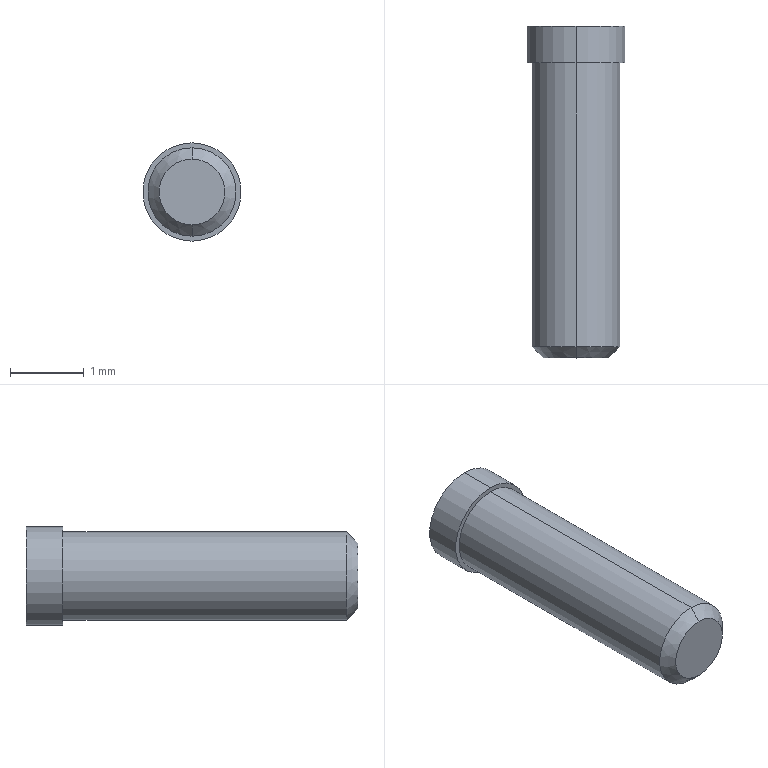Part | STEP file | MG_P_Screw_9_N | 1 solid | 16 faces | box 1.333 x 4.5 x 1.333 mm | volume 5.111 mm3 | plane 10 | cylinder 4 | cone 2 | commonest cylinder face diameters 1.2 x2 1.333 x2
STEP:
#1=CARTESIAN_POINT('',(0.,0.,0.));
#2=DIRECTION('',(0.,0.,1.));
#3=DIRECTION('',(1.,0.,0.));
#4=AXIS2_PLACEMENT_3D('',#1,#2,#3);
#5=CARTESIAN_POINT('',(0.,-4.,0.4465));
#6=VERTEX_POINT('',#5);
#7=CARTESIAN_POINT('',(0.,-4.,-0.4465));
#8=VERTEX_POINT('',#7);
#9=CARTESIAN_POINT('',(0.,-4.,0.));
#10=DIRECTION('',(0.,1.,0.));
#11=DIRECTION('',(0.,0.,1.));
#12=AXIS2_PLACEMENT_3D('',#9,#10,#11);
#13=CIRCLE('',#12,0.4465);
#14=CARTESIAN_POINT('',(0.,-4.,0.));
#15=DIRECTION('',(0.,1.,0.));
#16=DIRECTION('',(0.,0.,1.));
#17=AXIS2_PLACEMENT_3D('',#14,#15,#16);
#18=CONICAL_SURFACE('',#17,0.4465,0.7854);
#19=CARTESIAN_POINT('',(0.,0.));
#20=DIRECTION('',(1.,0.));
#21=VECTOR('',#20,1.);
#22=LINE('',#19,#21);
#23=(GEOMETRIC_REPRESENTATION_CONTEXT(2)PARAMETRIC_REPRESENTATION_CONTEXT()REPRESENTATION_CONTEXT('',''));
#24=DEFINITIONAL_REPRESENTATION('',(#22),#23);
#25=PCURVE('',#18,#24);
#26=CARTESIAN_POINT('',(0.4465,-4.,0.));
#27=DIRECTION('',(0.,1.,0.));
#28=DIRECTION('',(0.,0.,1.));
#29=AXIS2_PLACEMENT_3D('',#26,#27,#28);
#30=PLANE('',#29);
#31=CARTESIAN_POINT('',(0.,-0.4465));
#32=DIRECTION('',(1.,0.));
#33=AXIS2_PLACEMENT_2D('',#31,#32);
#34=CIRCLE('',#33,0.4465);
#35=(GEOMETRIC_REPRESENTATION_CONTEXT(2)PARAMETRIC_REPRESENTATION_CONTEXT()REPRESENTATION_CONTEXT('',''));
#36=DEFINITIONAL_REPRESENTATION('',(#34),#35);
#37=PCURVE('',#30,#36);
#38=SURFACE_CURVE('',#13,(#25,#37),.PCURVE_S1.);
#39=EDGE_CURVE('',#6,#8,#38,.T.);
#40=ORIENTED_EDGE('',*,*,#39,.T.);
#41=CARTESIAN_POINT('',(0.,-3.846,-0.6));
#42=VERTEX_POINT('',#41);
#43=CARTESIAN_POINT('',(0.,-4.,-0.4465));
#44=DIRECTION('',(0.,0.7071,-0.7071));
#45=VECTOR('',#44,1.);
#46=LINE('',#43,#45);
#47=CARTESIAN_POINT('',(3.142,0.));
#48=DIRECTION('',(0.,1.));
#49=VECTOR('',#48,1.);
#50=LINE('',#47,#49);
#51=(GEOMETRIC_REPRESENTATION_CONTEXT(2)PARAMETRIC_REPRESENTATION_CONTEXT()REPRESENTATION_CONTEXT('',''));
#52=DEFINITIONAL_REPRESENTATION('',(#50),#51);
#53=PCURVE('',#18,#52);
#54=CARTESIAN_POINT('',(0.,-4.,0.));
#55=DIRECTION('',(0.,1.,0.));
#56=DIRECTION('',(0.,0.,1.));
#57=AXIS2_PLACEMENT_3D('',#54,#55,#56);
#58=CONICAL_SURFACE('',#57,0.4465,0.7854);
#59=CARTESIAN_POINT('',(3.142,0.));
#60=DIRECTION('',(0.,1.));
#61=VECTOR('',#60,1.);
#62=LINE('',#59,#61);
#63=(GEOMETRIC_REPRESENTATION_CONTEXT(2)PARAMETRIC_REPRESENTATION_CONTEXT()REPRESENTATION_CONTEXT('',''));
#64=DEFINITIONAL_REPRESENTATION('',(#62),#63);
#65=PCURVE('',#58,#64);
#66=SURFACE_CURVE('',#46,(#53,#65),.PCURVE_S1.);
#67=EDGE_CURVE('',#8,#42,#66,.T.);
#68=ORIENTED_EDGE('',*,*,#67,.T.);
#69=CARTESIAN_POINT('',(0.,-3.846,0.6));
#70=VERTEX_POINT('',#69);
#71=CARTESIAN_POINT('',(0.,-3.846,0.));
#72=DIRECTION('',(0.,1.,0.));
#73=DIRECTION('',(0.,0.,1.));
#74=AXIS2_PLACEMENT_3D('',#71,#72,#73);
#75=CIRCLE('',#74,0.6);
#76=CARTESIAN_POINT('',(0.,0.1535));
#77=DIRECTION('',(1.,0.));
#78=VECTOR('',#77,1.);
#79=LINE('',#76,#78);
#80=(GEOMETRIC_REPRESENTATION_CONTEXT(2)PARAMETRIC_REPRESENTATION_CONTEXT()REPRESENTATION_CONTEXT('',''));
#81=DEFINITIONAL_REPRESENTATION('',(#79),#80);
#82=PCURVE('',#18,#81);
#83=CARTESIAN_POINT('',(0.,-4.,0.));
#84=DIRECTION('',(0.,1.,0.));
#85=DIRECTION('',(0.,0.,1.));
#86=AXIS2_PLACEMENT_3D('',#83,#84,#85);
#87=CYLINDRICAL_SURFACE('',#86,0.6);
#88=CARTESIAN_POINT('',(0.,0.1535));
#89=DIRECTION('',(1.,0.));
#90=VECTOR('',#89,1.);
#91=LINE('',#88,#90);
#92=(GEOMETRIC_REPRESENTATION_CONTEXT(2)PARAMETRIC_REPRESENTATION_CONTEXT()REPRESENTATION_CONTEXT('',''));
#93=DEFINITIONAL_REPRESENTATION('',(#91),#92);
#94=PCURVE('',#87,#93);
#95=SURFACE_CURVE('',#75,(#82,#94),.PCURVE_S1.);
#96=EDGE_CURVE('',#70,#42,#95,.T.);
#97=ORIENTED_EDGE('',*,*,#96,.F.);
#98=CARTESIAN_POINT('',(0.,-4.,0.4465));
#99=DIRECTION('',(0.,0.7071,0.7071));
#100=VECTOR('',#99,1.);
#101=LINE('',#98,#100);
#102=CARTESIAN_POINT('',(0.,0.));
#103=DIRECTION('',(0.,1.));
#104=VECTOR('',#103,1.);
#105=LINE('',#102,#104);
#106=(GEOMETRIC_REPRESENTATION_CONTEXT(2)PARAMETRIC_REPRESENTATION_CONTEXT()REPRESENTATION_CONTEXT('',''));
#107=DEFINITIONAL_REPRESENTATION('',(#105),#106);
#108=PCURVE('',#18,#107);
#109=CARTESIAN_POINT('',(6.283,0.));
#110=DIRECTION('',(0.,1.));
#111=VECTOR('',#110,1.);
#112=LINE('',#109,#111);
#113=(GEOMETRIC_REPRESENTATION_CONTEXT(2)PARAMETRIC_REPRESENTATION_CONTEXT()REPRESENTATION_CONTEXT('',''));
#114=DEFINITIONAL_REPRESENTATION('',(#112),#113);
#115=PCURVE('',#58,#114);
#116=SURFACE_CURVE('',#101,(#108,#115),.PCURVE_S1.);
#117=EDGE_CURVE('',#6,#70,#116,.T.);
#118=ORIENTED_EDGE('',*,*,#117,.F.);
#119=EDGE_LOOP('',(#40,#68,#97,#118));
#120=FACE_BOUND('',#119,.T.);
#121=ADVANCED_FACE('',(#120),#18,.T.);
#122=ORIENTED_EDGE('',*,*,#96,.T.);
#123=CARTESIAN_POINT('',(0.,0.,-0.6));
#124=VERTEX_POINT('',#123);
#125=CARTESIAN_POINT('',(0.,-4.,-0.6));
#126=DIRECTION('',(0.,1.,0.));
#127=VECTOR('',#126,1.);
#128=LINE('',#125,#127);
#129=CARTESIAN_POINT('',(3.142,0.));
#130=DIRECTION('',(0.,1.));
#131=VECTOR('',#130,1.);
#132=LINE('',#129,#131);
#133=(GEOMETRIC_REPRESENTATION_CONTEXT(2)PARAMETRIC_REPRESENTATION_CONTEXT()REPRESENTATION_CONTEXT('',''));
#134=DEFINITIONAL_REPRESENTATION('',(#132),#133);
#135=PCURVE('',#87,#134);
#136=CARTESIAN_POINT('',(0.,-4.,0.));
#137=DIRECTION('',(0.,1.,0.));
#138=DIRECTION('',(0.,0.,1.));
#139=AXIS2_PLACEMENT_3D('',#136,#137,#138);
#140=CYLINDRICAL_SURFACE('',#139,0.6);
#141=CARTESIAN_POINT('',(3.142,0.));
#142=DIRECTION('',(0.,1.));
#143=VECTOR('',#142,1.);
#144=LINE('',#141,#143);
#145=(GEOMETRIC_REPRESENTATION_CONTEXT(2)PARAMETRIC_REPRESENTATION_CONTEXT()REPRESENTATION_CONTEXT('',''));
#146=DEFINITIONAL_REPRESENTATION('',(#144),#145);
#147=PCURVE('',#140,#146);
#148=SURFACE_CURVE('',#128,(#135,#147),.PCURVE_S1.);
#149=EDGE_CURVE('',#42,#124,#148,.T.);
#150=ORIENTED_EDGE('',*,*,#149,.T.);
#151=CARTESIAN_POINT('',(0.,0.,0.6));
#152=VERTEX_POINT('',#151);
#153=CARTESIAN_POINT('',(0.,0.,0.));
#154=DIRECTION('',(0.,1.,0.));
#155=DIRECTION('',(0.,0.,1.));
#156=AXIS2_PLACEMENT_3D('',#153,#154,#155);
#157=CIRCLE('',#156,0.6);
#158=CARTESIAN_POINT('',(0.,4.));
#159=DIRECTION('',(1.,0.));
#160=VECTOR('',#159,1.);
#161=LINE('',#158,#160);
#162=(GEOMETRIC_REPRESENTATION_CONTEXT(2)PARAMETRIC_REPRESENTATION_CONTEXT()REPRESENTATION_CONTEXT('',''));
#163=DEFINITIONAL_REPRESENTATION('',(#161),#162);
#164=PCURVE('',#87,#163);
#165=CARTESIAN_POINT('',(0.6667,0.,0.));
#166=DIRECTION('',(0.,1.,0.));
#167=DIRECTION('',(0.,0.,1.));
#168=AXIS2_PLACEMENT_3D('',#165,#166,#167);
#169=PLANE('',#168);
#170=CARTESIAN_POINT('',(0.,-0.6667));
#171=DIRECTION('',(1.,0.));
#172=AXIS2_PLACEMENT_2D('',#170,#171);
#173=CIRCLE('',#172,0.6);
#174=(GEOMETRIC_REPRESENTATION_CONTEXT(2)PARAMETRIC_REPRESENTATION_CONTEXT()REPRESENTATION_CONTEXT('',''));
#175=DEFINITIONAL_REPRESENTATION('',(#173),#174);
#176=PCURVE('',#169,#175);
#177=SURFACE_CURVE('',#157,(#164,#176),.PCURVE_S1.);
#178=EDGE_CURVE('',#152,#124,#177,.T.);
#179=ORIENTED_EDGE('',*,*,#178,.F.);
#180=CARTESIAN_POINT('',(0.,-4.,0.6));
#181=DIRECTION('',(0.,1.,0.));
#182=VECTOR('',#181,1.);
#183=LINE('',#180,#182);
#184=CARTESIAN_POINT('',(0.,0.));
#185=DIRECTION('',(0.,1.));
#186=VECTOR('',#185,1.);
#187=LINE('',#184,#186);
#188=(GEOMETRIC_REPRESENTATION_CONTEXT(2)PARAMETRIC_REPRESENTATION_CONTEXT()REPRESENTATION_CONTEXT('',''));
#189=DEFINITIONAL_REPRESENTATION('',(#187),#188);
#190=PCURVE('',#87,#189);
#191=CARTESIAN_POINT('',(6.283,0.));
#192=DIRECTION('',(0.,1.));
#193=VECTOR('',#192,1.);
#194=LINE('',#191,#193);
#195=(GEOMETRIC_REPRESENTATION_CONTEXT(2)PARAMETRIC_REPRESENTATION_CONTEXT()REPRESENTATION_CONTEXT('',''));
#196=DEFINITIONAL_REPRESENTATION('',(#194),#195);
#197=PCURVE('',#140,#196);
#198=SURFACE_CURVE('',#183,(#190,#197),.PCURVE_S1.);
#199=EDGE_CURVE('',#70,#152,#198,.T.);
#200=ORIENTED_EDGE('',*,*,#199,.F.);
#201=EDGE_LOOP('',(#122,#150,#179,#200));
#202=FACE_BOUND('',#201,.T.);
#203=ADVANCED_FACE('',(#202),#87,.T.);
#204=CARTESIAN_POINT('',(0.,0.,0.6667));
#205=VERTEX_POINT('',#204);
#206=CARTESIAN_POINT('',(0.,0.,-0.6667));
#207=VERTEX_POINT('',#206);
#208=CARTESIAN_POINT('',(0.,0.,0.));
#209=DIRECTION('',(0.,1.,0.));
#210=DIRECTION('',(0.,0.,1.));
#211=AXIS2_PLACEMENT_3D('',#208,#209,#210);
#212=CIRCLE('',#211,0.6667);
#213=CARTESIAN_POINT('',(0.,-4.,0.));
#214=DIRECTION('',(0.,1.,0.));
#215=DIRECTION('',(0.,0.,1.));
#216=AXIS2_PLACEMENT_3D('',#213,#214,#215);
#217=CYLINDRICAL_SURFACE('',#216,0.6667);
#218=CARTESIAN_POINT('',(0.,4.));
#219=DIRECTION('',(1.,0.));
#220=VECTOR('',#219,1.);
#221=LINE('',#218,#220);
#222=(GEOMETRIC_REPRESENTATION_CONTEXT(2)PARAMETRIC_REPRESENTATION_CONTEXT()REPRESENTATION_CONTEXT('',''));
#223=DEFINITIONAL_REPRESENTATION('',(#221),#222);
#224=PCURVE('',#217,#223);
#225=CARTESIAN_POINT('',(0.,-0.6667));
#226=DIRECTION('',(1.,0.));
#227=AXIS2_PLACEMENT_2D('',#225,#226);
#228=CIRCLE('',#227,0.6667);
#229=(GEOMETRIC_REPRESENTATION_CONTEXT(2)PARAMETRIC_REPRESENTATION_CONTEXT()REPRESENTATION_CONTEXT('',''));
#230=DEFINITIONAL_REPRESENTATION('',(#228),#229);
#231=PCURVE('',#169,#230);
#232=SURFACE_CURVE('',#212,(#224,#231),.PCURVE_S1.);
#233=EDGE_CURVE('',#205,#207,#232,.T.);
#234=ORIENTED_EDGE('',*,*,#233,.T.);
#235=CARTESIAN_POINT('',(0.,0.5,-0.6667));
#236=VERTEX_POINT('',#235);
#237=CARTESIAN_POINT('',(0.,-4.,-0.6667));
#238=DIRECTION('',(0.,1.,0.));
#239=VECTOR('',#238,1.);
#240=LINE('',#237,#239);
#241=CARTESIAN_POINT('',(3.142,0.));
#242=DIRECTION('',(0.,1.));
#243=VECTOR('',#242,1.);
#244=LINE('',#241,#243);
#245=(GEOMETRIC_REPRESENTATION_CONTEXT(2)PARAMETRIC_REPRESENTATION_CONTEXT()REPRESENTATION_CONTEXT('',''));
#246=DEFINITIONAL_REPRESENTATION('',(#244),#245);
#247=PCURVE('',#217,#246);
#248=CARTESIAN_POINT('',(0.,-4.,0.));
#249=DIRECTION('',(0.,1.,0.));
#250=DIRECTION('',(0.,0.,1.));
#251=AXIS2_PLACEMENT_3D('',#248,#249,#250);
#252=CYLINDRICAL_SURFACE('',#251,0.6667);
#253=CARTESIAN_POINT('',(3.142,0.));
#254=DIRECTION('',(0.,1.));
#255=VECTOR('',#254,1.);
#256=LINE('',#253,#255);
#257=(GEOMETRIC_REPRESENTATION_CONTEXT(2)PARAMETRIC_REPRESENTATION_CONTEXT()REPRESENTATION_CONTEXT('',''));
#258=DEFINITIONAL_REPRESENTATION('',(#256),#257);
#259=PCURVE('',#252,#258);
#260=SURFACE_CURVE('',#240,(#247,#259),.PCURVE_S1.);
#261=EDGE_CURVE('',#207,#236,#260,.T.);
#262=ORIENTED_EDGE('',*,*,#261,.T.);
#263=CARTESIAN_POINT('',(0.,0.5,0.6667));
#264=VERTEX_POINT('',#263);
#265=CARTESIAN_POINT('',(0.,0.5,0.));
#266=DIRECTION('',(0.,1.,0.));
#267=DIRECTION('',(0.,0.,1.));
#268=AXIS2_PLACEMENT_3D('',#265,#266,#267);
#269=CIRCLE('',#268,0.6667);
#270=CARTESIAN_POINT('',(0.,4.5));
#271=DIRECTION('',(1.,0.));
#272=VECTOR('',#271,1.);
#273=LINE('',#270,#272);
#274=(GEOMETRIC_REPRESENTATION_CONTEXT(2)PARAMETRIC_REPRESENTATION_CONTEXT()REPRESENTATION_CONTEXT('',''));
#275=DEFINITIONAL_REPRESENTATION('',(#273),#274);
#276=PCURVE('',#217,#275);
#277=CARTESIAN_POINT('',(0.,0.5,0.));
#278=DIRECTION('',(0.,-1.,0.));
#279=DIRECTION('',(0.,0.,-1.));
#280=AXIS2_PLACEMENT_3D('',#277,#278,#279);
#281=PLANE('',#280);
#282=CARTESIAN_POINT('',(-0.6667,0.));
#283=CARTESIAN_POINT('',(-0.6667,1.155));
#284=CARTESIAN_POINT('',(0.3333,0.5774));
#285=CARTESIAN_POINT('',(1.333,0.));
#286=CARTESIAN_POINT('',(0.3333,-0.5774));
#287=CARTESIAN_POINT('',(-0.6667,-1.155));
#288=CARTESIAN_POINT('',(-0.6667,0.));
#289=(BOUNDED_CURVE()B_SPLINE_CURVE(2,(#282,#283,#284,#285,#286,#287,#288),.UNSPECIFIED.,.T.,.F.)B_SPLINE_CURVE_WITH_KNOTS((1,2,2,2,2,1),(-2.094,0.,2.094,4.189,6.283,8.378),.UNSPECIFIED.)CURVE()GEOMETRIC_REPRESENTATION_ITEM()RATIONAL_B_SPLINE_CURVE((1.,0.5,1.,0.5,1.,0.5,1.))REPRESENTATION_ITEM(''));
#290=(GEOMETRIC_REPRESENTATION_CONTEXT(2)PARAMETRIC_REPRESENTATION_CONTEXT()REPRESENTATION_CONTEXT('',''));
#291=DEFINITIONAL_REPRESENTATION('',(#289),#290);
#292=PCURVE('',#281,#291);
#293=SURFACE_CURVE('',#269,(#276,#292),.PCURVE_S1.);
#294=EDGE_CURVE('',#264,#236,#293,.T.);
#295=ORIENTED_EDGE('',*,*,#294,.F.);
#296=CARTESIAN_POINT('',(0.,-4.,0.6667));
#297=DIRECTION('',(0.,1.,0.));
#298=VECTOR('',#297,1.);
#299=LINE('',#296,#298);
#300=CARTESIAN_POINT('',(0.,0.));
#301=DIRECTION('',(0.,1.));
#302=VECTOR('',#301,1.);
#303=LINE('',#300,#302);
#304=(GEOMETRIC_REPRESENTATION_CONTEXT(2)PARAMETRIC_REPRESENTATION_CONTEXT()REPRESENTATION_CONTEXT('',''));
#305=DEFINITIONAL_REPRESENTATION('',(#303),#304);
#306=PCURVE('',#217,#305);
#307=CARTESIAN_POINT('',(6.283,0.));
#308=DIRECTION('',(0.,1.));
#309=VECTOR('',#308,1.);
#310=LINE('',#307,#309);
#311=(GEOMETRIC_REPRESENTATION_CONTEXT(2)PARAMETRIC_REPRESENTATION_CONTEXT()REPRESENTATION_CONTEXT('',''));
#312=DEFINITIONAL_REPRESENTATION('',(#310),#311);
#313=PCURVE('',#252,#312);
#314=SURFACE_CURVE('',#299,(#306,#313),.PCURVE_S1.);
#315=EDGE_CURVE('',#205,#264,#314,.T.);
#316=ORIENTED_EDGE('',*,*,#315,.F.);
#317=EDGE_LOOP('',(#234,#262,#295,#316));
#318=FACE_BOUND('',#317,.T.);
#319=ADVANCED_FACE('',(#318),#217,.T.);
#320=CARTESIAN_POINT('',(-0.2857,0.5,0.165));
#321=VERTEX_POINT('',#320);
#322=CARTESIAN_POINT('',(0.,0.5,0.3299));
#323=VERTEX_POINT('',#322);
#324=CARTESIAN_POINT('',(-0.2857,0.5,0.165));
#325=DIRECTION('',(0.866,0.,0.5));
#326=VECTOR('',#325,1.);
#327=LINE('',#324,#326);
#328=CARTESIAN_POINT('',(-0.165,-0.2857));
#329=DIRECTION('',(-0.5,0.866));
#330=VECTOR('',#329,1.);
#331=LINE('',#328,#330);
#332=(GEOMETRIC_REPRESENTATION_CONTEXT(2)PARAMETRIC_REPRESENTATION_CONTEXT()REPRESENTATION_CONTEXT('',''));
#333=DEFINITIONAL_REPRESENTATION('',(#331),#332);
#334=PCURVE('',#281,#333);
#335=CARTESIAN_POINT('',(-0.2857,0.25,0.165));
#336=DIRECTION('',(-0.5,0.,0.866));
#337=DIRECTION('',(0.866,0.,0.5));
#338=AXIS2_PLACEMENT_3D('',#335,#336,#337);
#339=PLANE('',#338);
#340=CARTESIAN_POINT('',(0.,0.25));
#341=DIRECTION('',(1.,0.));
#342=VECTOR('',#341,1.);
#343=LINE('',#340,#342);
#344=(GEOMETRIC_REPRESENTATION_CONTEXT(2)PARAMETRIC_REPRESENTATION_CONTEXT()REPRESENTATION_CONTEXT('',''));
#345=DEFINITIONAL_REPRESENTATION('',(#343),#344);
#346=PCURVE('',#339,#345);
#347=SURFACE_CURVE('',#327,(#334,#346),.PCURVE_S1.);
#348=EDGE_CURVE('',#321,#323,#347,.T.);
#349=ORIENTED_EDGE('',*,*,#348,.F.);
#350=CARTESIAN_POINT('',(-0.2857,0.5,-0.165));
#351=VERTEX_POINT('',#350);
#352=CARTESIAN_POINT('',(-0.2857,0.5,-0.165));
#353=DIRECTION('',(0.,0.,1.));
#354=VECTOR('',#353,1.);
#355=LINE('',#352,#354);
#356=CARTESIAN_POINT('',(0.165,-0.2857));
#357=DIRECTION('',(-1.,0.));
#358=VECTOR('',#357,1.);
#359=LINE('',#356,#358);
#360=(GEOMETRIC_REPRESENTATION_CONTEXT(2)PARAMETRIC_REPRESENTATION_CONTEXT()REPRESENTATION_CONTEXT('',''));
#361=DEFINITIONAL_REPRESENTATION('',(#359),#360);
#362=PCURVE('',#281,#361);
#363=CARTESIAN_POINT('',(-0.2857,0.25,-0.165));
#364=DIRECTION('',(-1.,0.,0.));
#365=DIRECTION('',(0.,0.,1.));
#366=AXIS2_PLACEMENT_3D('',#363,#364,#365);
#367=PLANE('',#366);
#368=CARTESIAN_POINT('',(0.,0.25));
#369=DIRECTION('',(1.,0.));
#370=VECTOR('',#369,1.);
#371=LINE('',#368,#370);
#372=(GEOMETRIC_REPRESENTATION_CONTEXT(2)PARAMETRIC_REPRESENTATION_CONTEXT()REPRESENTATION_CONTEXT('',''));
#373=DEFINITIONAL_REPRESENTATION('',(#371),#372);
#374=PCURVE('',#367,#373);
#375=SURFACE_CURVE('',#355,(#362,#374),.PCURVE_S1.);
#376=EDGE_CURVE('',#351,#321,#375,.T.);
#377=ORIENTED_EDGE('',*,*,#376,.F.);
#378=CARTESIAN_POINT('',(0.,0.5,-0.3299));
#379=VERTEX_POINT('',#378);
#380=CARTESIAN_POINT('',(0.,0.5,-0.3299));
#381=DIRECTION('',(-0.866,0.,0.5));
#382=VECTOR('',#381,1.);
#383=LINE('',#380,#382);
#384=CARTESIAN_POINT('',(0.3299,0.));
#385=DIRECTION('',(-0.5,-0.866));
#386=VECTOR('',#385,1.);
#387=LINE('',#384,#386);
#388=(GEOMETRIC_REPRESENTATION_CONTEXT(2)PARAMETRIC_REPRESENTATION_CONTEXT()REPRESENTATION_CONTEXT('',''));
#389=DEFINITIONAL_REPRESENTATION('',(#387),#388);
#390=PCURVE('',#281,#389);
#391=CARTESIAN_POINT('',(0.,0.25,-0.3299));
#392=DIRECTION('',(-0.5,0.,-0.866));
#393=DIRECTION('',(-0.866,0.,0.5));
#394=AXIS2_PLACEMENT_3D('',#391,#392,#393);
#395=PLANE('',#394);
#396=CARTESIAN_POINT('',(0.,0.25));
#397=DIRECTION('',(1.,0.));
#398=VECTOR('',#397,1.);
#399=LINE('',#396,#398);
#400=(GEOMETRIC_REPRESENTATION_CONTEXT(2)PARAMETRIC_REPRESENTATION_CONTEXT()REPRESENTATION_CONTEXT('',''));
#401=DEFINITIONAL_REPRESENTATION('',(#399),#400);
#402=PCURVE('',#395,#401);
#403=SURFACE_CURVE('',#383,(#390,#402),.PCURVE_S1.);
#404=EDGE_CURVE('',#379,#351,#403,.T.);
#405=ORIENTED_EDGE('',*,*,#404,.F.);
#406=CARTESIAN_POINT('',(0.2857,0.5,-0.165));
#407=VERTEX_POINT('',#406);
#408=CARTESIAN_POINT('',(0.2857,0.5,-0.165));
#409=DIRECTION('',(-0.866,0.,-0.5));
#410=VECTOR('',#409,1.);
#411=LINE('',#408,#410);
#412=CARTESIAN_POINT('',(0.165,0.2857));
#413=DIRECTION('',(0.5,-0.866));
#414=VECTOR('',#413,1.);
#415=LINE('',#412,#414);
#416=(GEOMETRIC_REPRESENTATION_CONTEXT(2)PARAMETRIC_REPRESENTATION_CONTEXT()REPRESENTATION_CONTEXT('',''));
#417=DEFINITIONAL_REPRESENTATION('',(#415),#416);
#418=PCURVE('',#281,#417);
#419=CARTESIAN_POINT('',(0.2857,0.25,-0.165));
#420=DIRECTION('',(0.5,0.,-0.866));
#421=DIRECTION('',(-0.866,0.,-0.5));
#422=AXIS2_PLACEMENT_3D('',#419,#420,#421);
#423=PLANE('',#422);
#424=CARTESIAN_POINT('',(0.,0.25));
#425=DIRECTION('',(1.,0.));
#426=VECTOR('',#425,1.);
#427=LINE('',#424,#426);
#428=(GEOMETRIC_REPRESENTATION_CONTEXT(2)PARAMETRIC_REPRESENTATION_CONTEXT()REPRESENTATION_CONTEXT('',''));
#429=DEFINITIONAL_REPRESENTATION('',(#427),#428);
#430=PCURVE('',#423,#429);
#431=SURFACE_CURVE('',#411,(#418,#430),.PCURVE_S1.);
#432=EDGE_CURVE('',#407,#379,#431,.T.);
#433=ORIENTED_EDGE('',*,*,#432,.F.);
#434=CARTESIAN_POINT('',(0.2857,0.5,0.165));
#435=VERTEX_POINT('',#434);
#436=CARTESIAN_POINT('',(0.2857,0.5,0.165));
#437=DIRECTION('',(0.,0.,-1.));
#438=VECTOR('',#437,1.);
#439=LINE('',#436,#438);
#440=CARTESIAN_POINT('',(-0.165,0.2857));
#441=DIRECTION('',(1.,0.));
#442=VECTOR('',#441,1.);
#443=LINE('',#440,#442);
#444=(GEOMETRIC_REPRESENTATION_CONTEXT(2)PARAMETRIC_REPRESENTATION_CONTEXT()REPRESENTATION_CONTEXT('',''));
#445=DEFINITIONAL_REPRESENTATION('',(#443),#444);
#446=PCURVE('',#281,#445);
#447=CARTESIAN_POINT('',(0.2857,0.25,0.165));
#448=DIRECTION('',(1.,0.,0.));
#449=DIRECTION('',(0.,0.,-1.));
#450=AXIS2_PLACEMENT_3D('',#447,#448,#449);
#451=PLANE('',#450);
#452=CARTESIAN_POINT('',(0.,0.25));
#453=DIRECTION('',(1.,0.));
#454=VECTOR('',#453,1.);
#455=LINE('',#452,#454);
#456=(GEOMETRIC_REPRESENTATION_CONTEXT(2)PARAMETRIC_REPRESENTATION_CONTEXT()REPRESENTATION_CONTEXT('',''));
#457=DEFINITIONAL_REPRESENTATION('',(#455),#456);
#458=PCURVE('',#451,#457);
#459=SURFACE_CURVE('',#439,(#446,#458),.PCURVE_S1.);
#460=EDGE_CURVE('',#435,#407,#459,.T.);
#461=ORIENTED_EDGE('',*,*,#460,.F.);
#462=CARTESIAN_POINT('',(0.,0.5,0.3299));
#463=DIRECTION('',(0.866,0.,-0.5));
#464=VECTOR('',#463,1.);
#465=LINE('',#462,#464);
#466=CARTESIAN_POINT('',(-0.3299,0.));
#467=DIRECTION('',(0.5,0.866));
#468=VECTOR('',#467,1.);
#469=LINE('',#466,#468);
#470=(GEOMETRIC_REPRESENTATION_CONTEXT(2)PARAMETRIC_REPRESENTATION_CONTEXT()REPRESENTATION_CONTEXT('',''));
#471=DEFINITIONAL_REPRESENTATION('',(#469),#470);
#472=PCURVE('',#281,#471);
#473=CARTESIAN_POINT('',(0.,0.25,0.3299));
#474=DIRECTION('',(0.5,0.,0.866));
#475=DIRECTION('',(0.866,0.,-0.5));
#476=AXIS2_PLACEMENT_3D('',#473,#474,#475);
#477=PLANE('',#476);
#478=CARTESIAN_POINT('',(0.,0.25));
#479=DIRECTION('',(1.,0.));
#480=VECTOR('',#479,1.);
#481=LINE('',#478,#480);
#482=(GEOMETRIC_REPRESENTATION_CONTEXT(2)PARAMETRIC_REPRESENTATION_CONTEXT()REPRESENTATION_CONTEXT('',''));
#483=DEFINITIONAL_REPRESENTATION('',(#481),#482);
#484=PCURVE('',#477,#483);
#485=SURFACE_CURVE('',#465,(#472,#484),.PCURVE_S1.);
#486=EDGE_CURVE('',#323,#435,#485,.T.);
#487=ORIENTED_EDGE('',*,*,#486,.F.);
#488=EDGE_LOOP('',(#349,#377,#405,#433,#461,#487));
#489=FACE_BOUND('',#488,.T.);
#490=ORIENTED_EDGE('',*,*,#294,.T.);
#491=CARTESIAN_POINT('',(0.,0.5,0.));
#492=DIRECTION('',(0.,1.,0.));
#493=DIRECTION('',(0.,0.,1.));
#494=AXIS2_PLACEMENT_3D('',#491,#492,#493);
#495=CIRCLE('',#494,0.6667);
#496=CARTESIAN_POINT('',(-0.6667,0.));
#497=CARTESIAN_POINT('',(-0.6667,1.155));
#498=CARTESIAN_POINT('',(0.3333,0.5774));
#499=CARTESIAN_POINT('',(1.333,0.));
#500=CARTESIAN_POINT('',(0.3333,-0.5774));
#501=CARTESIAN_POINT('',(-0.6667,-1.155));
#502=CARTESIAN_POINT('',(-0.6667,0.));
#503=(BOUNDED_CURVE()B_SPLINE_CURVE(2,(#496,#497,#498,#499,#500,#501,#502),.UNSPECIFIED.,.T.,.F.)B_SPLINE_CURVE_WITH_KNOTS((1,2,2,2,2,1),(-2.094,0.,2.094,4.189,6.283,8.378),.UNSPECIFIED.)CURVE()GEOMETRIC_REPRESENTATION_ITEM()RATIONAL_B_SPLINE_CURVE((1.,0.5,1.,0.5,1.,0.5,1.))REPRESENTATION_ITEM(''));
#504=(GEOMETRIC_REPRESENTATION_CONTEXT(2)PARAMETRIC_REPRESENTATION_CONTEXT()REPRESENTATION_CONTEXT('',''));
#505=DEFINITIONAL_REPRESENTATION('',(#503),#504);
#506=PCURVE('',#281,#505);
#507=CARTESIAN_POINT('',(0.,4.5));
#508=DIRECTION('',(1.,0.));
#509=VECTOR('',#508,1.);
#510=LINE('',#507,#509);
#511=(GEOMETRIC_REPRESENTATION_CONTEXT(2)PARAMETRIC_REPRESENTATION_CONTEXT()REPRESENTATION_CONTEXT('',''));
#512=DEFINITIONAL_REPRESENTATION('',(#510),#511);
#513=PCURVE('',#252,#512);
#514=SURFACE_CURVE('',#495,(#506,#513),.PCURVE_S1.);
#515=EDGE_CURVE('',#236,#264,#514,.T.);
#516=ORIENTED_EDGE('',*,*,#515,.T.);
#517=EDGE_LOOP('',(#490,#516));
#518=FACE_BOUND('',#517,.T.);
#519=ADVANCED_FACE('',(#489,#518),#281,.F.);
#520=ORIENTED_EDGE('',*,*,#261,.F.);
#521=CARTESIAN_POINT('',(0.,0.,0.));
#522=DIRECTION('',(0.,1.,0.));
#523=DIRECTION('',(0.,0.,1.));
#524=AXIS2_PLACEMENT_3D('',#521,#522,#523);
#525=CIRCLE('',#524,0.6667);
#526=CARTESIAN_POINT('',(0.,4.));
#527=DIRECTION('',(1.,0.));
#528=VECTOR('',#527,1.);
#529=LINE('',#526,#528);
#530=(GEOMETRIC_REPRESENTATION_CONTEXT(2)PARAMETRIC_REPRESENTATION_CONTEXT()REPRESENTATION_CONTEXT('',''));
#531=DEFINITIONAL_REPRESENTATION('',(#529),#530);
#532=PCURVE('',#252,#531);
#533=CARTESIAN_POINT('',(0.,-0.6667));
#534=DIRECTION('',(1.,0.));
#535=AXIS2_PLACEMENT_2D('',#533,#534);
#536=CIRCLE('',#535,0.6667);
#537=(GEOMETRIC_REPRESENTATION_CONTEXT(2)PARAMETRIC_REPRESENTATION_CONTEXT()REPRESENTATION_CONTEXT('',''));
#538=DEFINITIONAL_REPRESENTATION('',(#536),#537);
#539=PCURVE('',#169,#538);
#540=SURFACE_CURVE('',#525,(#532,#539),.PCURVE_S1.);
#541=EDGE_CURVE('',#207,#205,#540,.T.);
#542=ORIENTED_EDGE('',*,*,#541,.T.);
#543=ORIENTED_EDGE('',*,*,#315,.T.);
#544=ORIENTED_EDGE('',*,*,#515,.F.);
#545=EDGE_LOOP('',(#520,#542,#543,#544));
#546=FACE_BOUND('',#545,.T.);
#547=ADVANCED_FACE('',(#546),#252,.T.);
#548=ORIENTED_EDGE('',*,*,#233,.F.);
#549=ORIENTED_EDGE('',*,*,#541,.F.);
#550=EDGE_LOOP('',(#548,#549));
#551=FACE_BOUND('',#550,.T.);
#552=ORIENTED_EDGE('',*,*,#178,.T.);
#553=CARTESIAN_POINT('',(0.,0.,0.));
#554=DIRECTION('',(0.,1.,0.));
#555=DIRECTION('',(0.,0.,1.));
#556=AXIS2_PLACEMENT_3D('',#553,#554,#555);
#557=CIRCLE('',#556,0.6);
#558=CARTESIAN_POINT('',(0.,-0.6667));
#559=DIRECTION('',(1.,0.));
#560=AXIS2_PLACEMENT_2D('',#558,#559);
#561=CIRCLE('',#560,0.6);
#562=(GEOMETRIC_REPRESENTATION_CONTEXT(2)PARAMETRIC_REPRESENTATION_CONTEXT()REPRESENTATION_CONTEXT('',''));
#563=DEFINITIONAL_REPRESENTATION('',(#561),#562);
#564=PCURVE('',#169,#563);
#565=CARTESIAN_POINT('',(0.,4.));
#566=DIRECTION('',(1.,0.));
#567=VECTOR('',#566,1.);
#568=LINE('',#565,#567);
#569=(GEOMETRIC_REPRESENTATION_CONTEXT(2)PARAMETRIC_REPRESENTATION_CONTEXT()REPRESENTATION_CONTEXT('',''));
#570=DEFINITIONAL_REPRESENTATION('',(#568),#569);
#571=PCURVE('',#140,#570);
#572=SURFACE_CURVE('',#557,(#564,#571),.PCURVE_S1.);
#573=EDGE_CURVE('',#124,#152,#572,.T.);
#574=ORIENTED_EDGE('',*,*,#573,.T.);
#575=EDGE_LOOP('',(#552,#574));
#576=FACE_BOUND('',#575,.T.);
#577=ADVANCED_FACE('',(#551,#576),#169,.F.);
#578=ORIENTED_EDGE('',*,*,#149,.F.);
#579=CARTESIAN_POINT('',(0.,-3.846,0.));
#580=DIRECTION('',(0.,1.,0.));
#581=DIRECTION('',(0.,0.,1.));
#582=AXIS2_PLACEMENT_3D('',#579,#580,#581);
#583=CIRCLE('',#582,0.6);
#584=CARTESIAN_POINT('',(0.,0.1535));
#585=DIRECTION('',(1.,0.));
#586=VECTOR('',#585,1.);
#587=LINE('',#584,#586);
#588=(GEOMETRIC_REPRESENTATION_CONTEXT(2)PARAMETRIC_REPRESENTATION_CONTEXT()REPRESENTATION_CONTEXT('',''));
#589=DEFINITIONAL_REPRESENTATION('',(#587),#588);
#590=PCURVE('',#140,#589);
#591=CARTESIAN_POINT('',(0.,0.1535));
#592=DIRECTION('',(1.,0.));
#593=VECTOR('',#592,1.);
#594=LINE('',#591,#593);
#595=(GEOMETRIC_REPRESENTATION_CONTEXT(2)PARAMETRIC_REPRESENTATION_CONTEXT()REPRESENTATION_CONTEXT('',''));
#596=DEFINITIONAL_REPRESENTATION('',(#594),#595);
#597=PCURVE('',#58,#596);
#598=SURFACE_CURVE('',#583,(#590,#597),.PCURVE_S1.);
#599=EDGE_CURVE('',#42,#70,#598,.T.);
#600=ORIENTED_EDGE('',*,*,#599,.T.);
#601=ORIENTED_EDGE('',*,*,#199,.T.);
#602=ORIENTED_EDGE('',*,*,#573,.F.);
#603=EDGE_LOOP('',(#578,#600,#601,#602));
#604=FACE_BOUND('',#603,.T.);
#605=ADVANCED_FACE('',(#604),#140,.T.);
#606=ORIENTED_EDGE('',*,*,#67,.F.);
#607=CARTESIAN_POINT('',(0.,-4.,0.));
#608=DIRECTION('',(0.,1.,0.));
#609=DIRECTION('',(0.,0.,1.));
#610=AXIS2_PLACEMENT_3D('',#607,#608,#609);
#611=CIRCLE('',#610,0.4465);
#612=CARTESIAN_POINT('',(0.,0.));
#613=DIRECTION('',(1.,0.));
#614=VECTOR('',#613,1.);
#615=LINE('',#612,#614);
#616=(GEOMETRIC_REPRESENTATION_CONTEXT(2)PARAMETRIC_REPRESENTATION_CONTEXT()REPRESENTATION_CONTEXT('',''));
#617=DEFINITIONAL_REPRESENTATION('',(#615),#616);
#618=PCURVE('',#58,#617);
#619=CARTESIAN_POINT('',(0.,-0.4465));
#620=DIRECTION('',(1.,0.));
#621=AXIS2_PLACEMENT_2D('',#619,#620);
#622=CIRCLE('',#621,0.4465);
#623=(GEOMETRIC_REPRESENTATION_CONTEXT(2)PARAMETRIC_REPRESENTATION_CONTEXT()REPRESENTATION_CONTEXT('',''));
#624=DEFINITIONAL_REPRESENTATION('',(#622),#623);
#625=PCURVE('',#30,#624);
#626=SURFACE_CURVE('',#611,(#618,#625),.PCURVE_S1.);
#627=EDGE_CURVE('',#8,#6,#626,.T.);
#628=ORIENTED_EDGE('',*,*,#627,.T.);
#629=ORIENTED_EDGE('',*,*,#117,.T.);
#630=ORIENTED_EDGE('',*,*,#599,.F.);
#631=EDGE_LOOP('',(#606,#628,#629,#630));
#632=FACE_BOUND('',#631,.T.);
#633=ADVANCED_FACE('',(#632),#58,.T.);
#634=ORIENTED_EDGE('',*,*,#39,.F.);
#635=ORIENTED_EDGE('',*,*,#627,.F.);
#636=EDGE_LOOP('',(#634,#635));
#637=FACE_BOUND('',#636,.T.);
#638=ADVANCED_FACE('',(#637),#30,.F.);
#639=ORIENTED_EDGE('',*,*,#376,.T.);
#640=CARTESIAN_POINT('',(-0.2857,0.25,0.165));
#641=VERTEX_POINT('',#640);
#642=CARTESIAN_POINT('',(-0.2857,0.25,0.165));
#643=DIRECTION('',(0.,1.,0.));
#644=VECTOR('',#643,1.);
#645=LINE('',#642,#644);
#646=CARTESIAN_POINT('',(0.3299,0.));
#647=DIRECTION('',(0.,1.));
#648=VECTOR('',#647,1.);
#649=LINE('',#646,#648);
#650=(GEOMETRIC_REPRESENTATION_CONTEXT(2)PARAMETRIC_REPRESENTATION_CONTEXT()REPRESENTATION_CONTEXT('',''));
#651=DEFINITIONAL_REPRESENTATION('',(#649),#650);
#652=PCURVE('',#367,#651);
#653=CARTESIAN_POINT('',(0.,0.));
#654=DIRECTION('',(0.,1.));
#655=VECTOR('',#654,1.);
#656=LINE('',#653,#655);
#657=(GEOMETRIC_REPRESENTATION_CONTEXT(2)PARAMETRIC_REPRESENTATION_CONTEXT()REPRESENTATION_CONTEXT('',''));
#658=DEFINITIONAL_REPRESENTATION('',(#656),#657);
#659=PCURVE('',#339,#658);
#660=SURFACE_CURVE('',#645,(#652,#659),.PCURVE_S1.);
#661=EDGE_CURVE('',#641,#321,#660,.T.);
#662=ORIENTED_EDGE('',*,*,#661,.F.);
#663=CARTESIAN_POINT('',(-0.2857,0.25,-0.165));
#664=VERTEX_POINT('',#663);
#665=CARTESIAN_POINT('',(-0.2857,0.25,-0.165));
#666=DIRECTION('',(0.,0.,1.));
#667=VECTOR('',#666,1.);
#668=LINE('',#665,#667);
#669=CARTESIAN_POINT('',(0.,0.));
#670=DIRECTION('',(1.,0.));
#671=VECTOR('',#670,1.);
#672=LINE('',#669,#671);
#673=(GEOMETRIC_REPRESENTATION_CONTEXT(2)PARAMETRIC_REPRESENTATION_CONTEXT()REPRESENTATION_CONTEXT('',''));
#674=DEFINITIONAL_REPRESENTATION('',(#672),#673);
#675=PCURVE('',#367,#674);
#676=CARTESIAN_POINT('',(0.,0.25,0.));
#677=DIRECTION('',(0.,1.,0.));
#678=DIRECTION('',(0.,0.,1.));
#679=AXIS2_PLACEMENT_3D('',#676,#677,#678);
#680=PLANE('',#679);
#681=CARTESIAN_POINT('',(-0.165,-0.2857));
#682=DIRECTION('',(1.,0.));
#683=VECTOR('',#682,1.);
#684=LINE('',#681,#683);
#685=(GEOMETRIC_REPRESENTATION_CONTEXT(2)PARAMETRIC_REPRESENTATION_CONTEXT()REPRESENTATION_CONTEXT('',''));
#686=DEFINITIONAL_REPRESENTATION('',(#684),#685);
#687=PCURVE('',#680,#686);
#688=SURFACE_CURVE('',#668,(#675,#687),.PCURVE_S1.);
#689=EDGE_CURVE('',#664,#641,#688,.T.);
#690=ORIENTED_EDGE('',*,*,#689,.F.);
#691=CARTESIAN_POINT('',(-0.2857,0.25,-0.165));
#692=DIRECTION('',(0.,1.,0.));
#693=VECTOR('',#692,1.);
#694=LINE('',#691,#693);
#695=CARTESIAN_POINT('',(0.,0.));
#696=DIRECTION('',(0.,1.));
#697=VECTOR('',#696,1.);
#698=LINE('',#695,#697);
#699=(GEOMETRIC_REPRESENTATION_CONTEXT(2)PARAMETRIC_REPRESENTATION_CONTEXT()REPRESENTATION_CONTEXT('',''));
#700=DEFINITIONAL_REPRESENTATION('',(#698),#699);
#701=PCURVE('',#367,#700);
#702=CARTESIAN_POINT('',(0.3299,0.));
#703=DIRECTION('',(0.,1.));
#704=VECTOR('',#703,1.);
#705=LINE('',#702,#704);
#706=(GEOMETRIC_REPRESENTATION_CONTEXT(2)PARAMETRIC_REPRESENTATION_CONTEXT()REPRESENTATION_CONTEXT('',''));
#707=DEFINITIONAL_REPRESENTATION('',(#705),#706);
#708=PCURVE('',#395,#707);
#709=SURFACE_CURVE('',#694,(#701,#708),.PCURVE_S1.);
#710=EDGE_CURVE('',#664,#351,#709,.T.);
#711=ORIENTED_EDGE('',*,*,#710,.T.);
#712=EDGE_LOOP('',(#639,#662,#690,#711));
#713=FACE_BOUND('',#712,.T.);
#714=ADVANCED_FACE('',(#713),#367,.F.);
#715=ORIENTED_EDGE('',*,*,#404,.T.);
#716=ORIENTED_EDGE('',*,*,#710,.F.);
#717=CARTESIAN_POINT('',(0.,0.25,-0.3299));
#718=VERTEX_POINT('',#717);
#719=CARTESIAN_POINT('',(0.,0.25,-0.3299));
#720=DIRECTION('',(-0.866,0.,0.5));
#721=VECTOR('',#720,1.);
#722=LINE('',#719,#721);
#723=CARTESIAN_POINT('',(0.,0.));
#724=DIRECTION('',(1.,0.));
#725=VECTOR('',#724,1.);
#726=LINE('',#723,#725);
#727=(GEOMETRIC_REPRESENTATION_CONTEXT(2)PARAMETRIC_REPRESENTATION_CONTEXT()REPRESENTATION_CONTEXT('',''));
#728=DEFINITIONAL_REPRESENTATION('',(#726),#727);
#729=PCURVE('',#395,#728);
#730=CARTESIAN_POINT('',(-0.3299,0.));
#731=DIRECTION('',(0.5,-0.866));
#732=VECTOR('',#731,1.);
#733=LINE('',#730,#732);
#734=(GEOMETRIC_REPRESENTATION_CONTEXT(2)PARAMETRIC_REPRESENTATION_CONTEXT()REPRESENTATION_CONTEXT('',''));
#735=DEFINITIONAL_REPRESENTATION('',(#733),#734);
#736=PCURVE('',#680,#735);
#737=SURFACE_CURVE('',#722,(#729,#736),.PCURVE_S1.);
#738=EDGE_CURVE('',#718,#664,#737,.T.);
#739=ORIENTED_EDGE('',*,*,#738,.F.);
#740=CARTESIAN_POINT('',(0.,0.25,-0.3299));
#741=DIRECTION('',(0.,1.,0.));
#742=VECTOR('',#741,1.);
#743=LINE('',#740,#742);
#744=CARTESIAN_POINT('',(0.,0.));
#745=DIRECTION('',(0.,1.));
#746=VECTOR('',#745,1.);
#747=LINE('',#744,#746);
#748=(GEOMETRIC_REPRESENTATION_CONTEXT(2)PARAMETRIC_REPRESENTATION_CONTEXT()REPRESENTATION_CONTEXT('',''));
#749=DEFINITIONAL_REPRESENTATION('',(#747),#748);
#750=PCURVE('',#395,#749);
#751=CARTESIAN_POINT('',(0.3299,0.));
#752=DIRECTION('',(0.,1.));
#753=VECTOR('',#752,1.);
#754=LINE('',#751,#753);
#755=(GEOMETRIC_REPRESENTATION_CONTEXT(2)PARAMETRIC_REPRESENTATION_CONTEXT()REPRESENTATION_CONTEXT('',''));
#756=DEFINITIONAL_REPRESENTATION('',(#754),#755);
#757=PCURVE('',#423,#756);
#758=SURFACE_CURVE('',#743,(#750,#757),.PCURVE_S1.);
#759=EDGE_CURVE('',#718,#379,#758,.T.);
#760=ORIENTED_EDGE('',*,*,#759,.T.);
#761=EDGE_LOOP('',(#715,#716,#739,#760));
#762=FACE_BOUND('',#761,.T.);
#763=ADVANCED_FACE('',(#762),#395,.F.);
#764=ORIENTED_EDGE('',*,*,#432,.T.);
#765=ORIENTED_EDGE('',*,*,#759,.F.);
#766=CARTESIAN_POINT('',(0.2857,0.25,-0.165));
#767=VERTEX_POINT('',#766);
#768=CARTESIAN_POINT('',(0.2857,0.25,-0.165));
#769=DIRECTION('',(-0.866,0.,-0.5));
#770=VECTOR('',#769,1.);
#771=LINE('',#768,#770);
#772=CARTESIAN_POINT('',(0.,0.));
#773=DIRECTION('',(1.,0.));
#774=VECTOR('',#773,1.);
#775=LINE('',#772,#774);
#776=(GEOMETRIC_REPRESENTATION_CONTEXT(2)PARAMETRIC_REPRESENTATION_CONTEXT()REPRESENTATION_CONTEXT('',''));
#777=DEFINITIONAL_REPRESENTATION('',(#775),#776);
#778=PCURVE('',#423,#777);
#779=CARTESIAN_POINT('',(-0.165,0.2857));
#780=DIRECTION('',(-0.5,-0.866));
#781=VECTOR('',#780,1.);
#782=LINE('',#779,#781);
#783=(GEOMETRIC_REPRESENTATION_CONTEXT(2)PARAMETRIC_REPRESENTATION_CONTEXT()REPRESENTATION_CONTEXT('',''));
#784=DEFINITIONAL_REPRESENTATION('',(#782),#783);
#785=PCURVE('',#680,#784);
#786=SURFACE_CURVE('',#771,(#778,#785),.PCURVE_S1.);
#787=EDGE_CURVE('',#767,#718,#786,.T.);
#788=ORIENTED_EDGE('',*,*,#787,.F.);
#789=CARTESIAN_POINT('',(0.2857,0.25,-0.165));
#790=DIRECTION('',(0.,1.,0.));
#791=VECTOR('',#790,1.);
#792=LINE('',#789,#791);
#793=CARTESIAN_POINT('',(0.,0.));
#794=DIRECTION('',(0.,1.));
#795=VECTOR('',#794,1.);
#796=LINE('',#793,#795);
#797=(GEOMETRIC_REPRESENTATION_CONTEXT(2)PARAMETRIC_REPRESENTATION_CONTEXT()REPRESENTATION_CONTEXT('',''));
#798=DEFINITIONAL_REPRESENTATION('',(#796),#797);
#799=PCURVE('',#423,#798);
#800=CARTESIAN_POINT('',(0.3299,0.));
#801=DIRECTION('',(0.,1.));
#802=VECTOR('',#801,1.);
#803=LINE('',#800,#802);
#804=(GEOMETRIC_REPRESENTATION_CONTEXT(2)PARAMETRIC_REPRESENTATION_CONTEXT()REPRESENTATION_CONTEXT('',''));
#805=DEFINITIONAL_REPRESENTATION('',(#803),#804);
#806=PCURVE('',#451,#805);
#807=SURFACE_CURVE('',#792,(#799,#806),.PCURVE_S1.);
#808=EDGE_CURVE('',#767,#407,#807,.T.);
#809=ORIENTED_EDGE('',*,*,#808,.T.);
#810=EDGE_LOOP('',(#764,#765,#788,#809));
#811=FACE_BOUND('',#810,.T.);
#812=ADVANCED_FACE('',(#811),#423,.F.);
#813=ORIENTED_EDGE('',*,*,#460,.T.);
#814=ORIENTED_EDGE('',*,*,#808,.F.);
#815=CARTESIAN_POINT('',(0.2857,0.25,0.165));
#816=VERTEX_POINT('',#815);
#817=CARTESIAN_POINT('',(0.2857,0.25,0.165));
#818=DIRECTION('',(0.,0.,-1.));
#819=VECTOR('',#818,1.);
#820=LINE('',#817,#819);
#821=CARTESIAN_POINT('',(0.,0.));
#822=DIRECTION('',(1.,0.));
#823=VECTOR('',#822,1.);
#824=LINE('',#821,#823);
#825=(GEOMETRIC_REPRESENTATION_CONTEXT(2)PARAMETRIC_REPRESENTATION_CONTEXT()REPRESENTATION_CONTEXT('',''));
#826=DEFINITIONAL_REPRESENTATION('',(#824),#825);
#827=PCURVE('',#451,#826);
#828=CARTESIAN_POINT('',(0.165,0.2857));
#829=DIRECTION('',(-1.,0.));
#830=VECTOR('',#829,1.);
#831=LINE('',#828,#830);
#832=(GEOMETRIC_REPRESENTATION_CONTEXT(2)PARAMETRIC_REPRESENTATION_CONTEXT()REPRESENTATION_CONTEXT('',''));
#833=DEFINITIONAL_REPRESENTATION('',(#831),#832);
#834=PCURVE('',#680,#833);
#835=SURFACE_CURVE('',#820,(#827,#834),.PCURVE_S1.);
#836=EDGE_CURVE('',#816,#767,#835,.T.);
#837=ORIENTED_EDGE('',*,*,#836,.F.);
#838=CARTESIAN_POINT('',(0.2857,0.25,0.165));
#839=DIRECTION('',(0.,1.,0.));
#840=VECTOR('',#839,1.);
#841=LINE('',#838,#840);
#842=CARTESIAN_POINT('',(0.,0.));
#843=DIRECTION('',(0.,1.));
#844=VECTOR('',#843,1.);
#845=LINE('',#842,#844);
#846=(GEOMETRIC_REPRESENTATION_CONTEXT(2)PARAMETRIC_REPRESENTATION_CONTEXT()REPRESENTATION_CONTEXT('',''));
#847=DEFINITIONAL_REPRESENTATION('',(#845),#846);
#848=PCURVE('',#451,#847);
#849=CARTESIAN_POINT('',(0.3299,0.));
#850=DIRECTION('',(0.,1.));
#851=VECTOR('',#850,1.);
#852=LINE('',#849,#851);
#853=(GEOMETRIC_REPRESENTATION_CONTEXT(2)PARAMETRIC_REPRESENTATION_CONTEXT()REPRESENTATION_CONTEXT('',''));
#854=DEFINITIONAL_REPRESENTATION('',(#852),#853);
#855=PCURVE('',#477,#854);
#856=SURFACE_CURVE('',#841,(#848,#855),.PCURVE_S1.);
#857=EDGE_CURVE('',#816,#435,#856,.T.);
#858=ORIENTED_EDGE('',*,*,#857,.T.);
#859=EDGE_LOOP('',(#813,#814,#837,#858));
#860=FACE_BOUND('',#859,.T.);
#861=ADVANCED_FACE('',(#860),#451,.F.);
#862=ORIENTED_EDGE('',*,*,#486,.T.);
#863=ORIENTED_EDGE('',*,*,#857,.F.);
#864=CARTESIAN_POINT('',(0.,0.25,0.3299));
#865=VERTEX_POINT('',#864);
#866=CARTESIAN_POINT('',(0.,0.25,0.3299));
#867=DIRECTION('',(0.866,0.,-0.5));
#868=VECTOR('',#867,1.);
#869=LINE('',#866,#868);
#870=CARTESIAN_POINT('',(0.,0.));
#871=DIRECTION('',(1.,0.));
#872=VECTOR('',#871,1.);
#873=LINE('',#870,#872);
#874=(GEOMETRIC_REPRESENTATION_CONTEXT(2)PARAMETRIC_REPRESENTATION_CONTEXT()REPRESENTATION_CONTEXT('',''));
#875=DEFINITIONAL_REPRESENTATION('',(#873),#874);
#876=PCURVE('',#477,#875);
#877=CARTESIAN_POINT('',(0.3299,0.));
#878=DIRECTION('',(-0.5,0.866));
#879=VECTOR('',#878,1.);
#880=LINE('',#877,#879);
#881=(GEOMETRIC_REPRESENTATION_CONTEXT(2)PARAMETRIC_REPRESENTATION_CONTEXT()REPRESENTATION_CONTEXT('',''));
#882=DEFINITIONAL_REPRESENTATION('',(#880),#881);
#883=PCURVE('',#680,#882);
#884=SURFACE_CURVE('',#869,(#876,#883),.PCURVE_S1.);
#885=EDGE_CURVE('',#865,#816,#884,.T.);
#886=ORIENTED_EDGE('',*,*,#885,.F.);
#887=CARTESIAN_POINT('',(0.,0.25,0.3299));
#888=DIRECTION('',(0.,1.,0.));
#889=VECTOR('',#888,1.);
#890=LINE('',#887,#889);
#891=CARTESIAN_POINT('',(0.,0.));
#892=DIRECTION('',(0.,1.));
#893=VECTOR('',#892,1.);
#894=LINE('',#891,#893);
#895=(GEOMETRIC_REPRESENTATION_CONTEXT(2)PARAMETRIC_REPRESENTATION_CONTEXT()REPRESENTATION_CONTEXT('',''));
#896=DEFINITIONAL_REPRESENTATION('',(#894),#895);
#897=PCURVE('',#477,#896);
#898=CARTESIAN_POINT('',(0.3299,0.));
#899=DIRECTION('',(0.,1.));
#900=VECTOR('',#899,1.);
#901=LINE('',#898,#900);
#902=(GEOMETRIC_REPRESENTATION_CONTEXT(2)PARAMETRIC_REPRESENTATION_CONTEXT()REPRESENTATION_CONTEXT('',''));
#903=DEFINITIONAL_REPRESENTATION('',(#901),#902);
#904=PCURVE('',#339,#903);
#905=SURFACE_CURVE('',#890,(#897,#904),.PCURVE_S1.);
#906=EDGE_CURVE('',#865,#323,#905,.T.);
#907=ORIENTED_EDGE('',*,*,#906,.T.);
#908=EDGE_LOOP('',(#862,#863,#886,#907));
#909=FACE_BOUND('',#908,.T.);
#910=ADVANCED_FACE('',(#909),#477,.F.);
#911=ORIENTED_EDGE('',*,*,#348,.T.);
#912=ORIENTED_EDGE('',*,*,#906,.F.);
#913=CARTESIAN_POINT('',(-0.2857,0.25,0.165));
#914=DIRECTION('',(0.866,0.,0.5));
#915=VECTOR('',#914,1.);
#916=LINE('',#913,#915);
#917=CARTESIAN_POINT('',(0.,0.));
#918=DIRECTION('',(1.,0.));
#919=VECTOR('',#918,1.);
#920=LINE('',#917,#919);
#921=(GEOMETRIC_REPRESENTATION_CONTEXT(2)PARAMETRIC_REPRESENTATION_CONTEXT()REPRESENTATION_CONTEXT('',''));
#922=DEFINITIONAL_REPRESENTATION('',(#920),#921);
#923=PCURVE('',#339,#922);
#924=CARTESIAN_POINT('',(0.165,-0.2857));
#925=DIRECTION('',(0.5,0.866));
#926=VECTOR('',#925,1.);
#927=LINE('',#924,#926);
#928=(GEOMETRIC_REPRESENTATION_CONTEXT(2)PARAMETRIC_REPRESENTATION_CONTEXT()REPRESENTATION_CONTEXT('',''));
#929=DEFINITIONAL_REPRESENTATION('',(#927),#928);
#930=PCURVE('',#680,#929);
#931=SURFACE_CURVE('',#916,(#923,#930),.PCURVE_S1.);
#932=EDGE_CURVE('',#641,#865,#931,.T.);
#933=ORIENTED_EDGE('',*,*,#932,.F.);
#934=ORIENTED_EDGE('',*,*,#661,.T.);
#935=EDGE_LOOP('',(#911,#912,#933,#934));
#936=FACE_BOUND('',#935,.T.);
#937=ADVANCED_FACE('',(#936),#339,.F.);
#938=ORIENTED_EDGE('',*,*,#689,.T.);
#939=ORIENTED_EDGE('',*,*,#932,.T.);
#940=ORIENTED_EDGE('',*,*,#885,.T.);
#941=ORIENTED_EDGE('',*,*,#836,.T.);
#942=ORIENTED_EDGE('',*,*,#787,.T.);
#943=ORIENTED_EDGE('',*,*,#738,.T.);
#944=EDGE_LOOP('',(#938,#939,#940,#941,#942,#943));
#945=FACE_BOUND('',#944,.T.);
#946=ADVANCED_FACE('',(#945),#680,.T.);
#947=CLOSED_SHELL('',(#121,#203,#319,#519,#547,#577,#605,#633,#638,#714,#763,#812,#861,#910,#937,#946));
#948=MANIFOLD_SOLID_BREP('',#947);
#949=(LENGTH_UNIT()NAMED_UNIT(*)SI_UNIT(.MILLI.,.METRE.));
#950=UNCERTAINTY_MEASURE_WITH_UNIT(LENGTH_MEASURE(0.0000001),#949,'','');
#951=(NAMED_UNIT(*)PLANE_ANGLE_UNIT()SI_UNIT($,.RADIAN.));
#952=(NAMED_UNIT(*)SI_UNIT($,.STERADIAN.)SOLID_ANGLE_UNIT());
#953=(GEOMETRIC_REPRESENTATION_CONTEXT(3)GLOBAL_UNCERTAINTY_ASSIGNED_CONTEXT((#950))GLOBAL_UNIT_ASSIGNED_CONTEXT((#949,#951,#952))REPRESENTATION_CONTEXT('',''));
#954=ADVANCED_BREP_SHAPE_REPRESENTATION('',(#4,#948),#953);